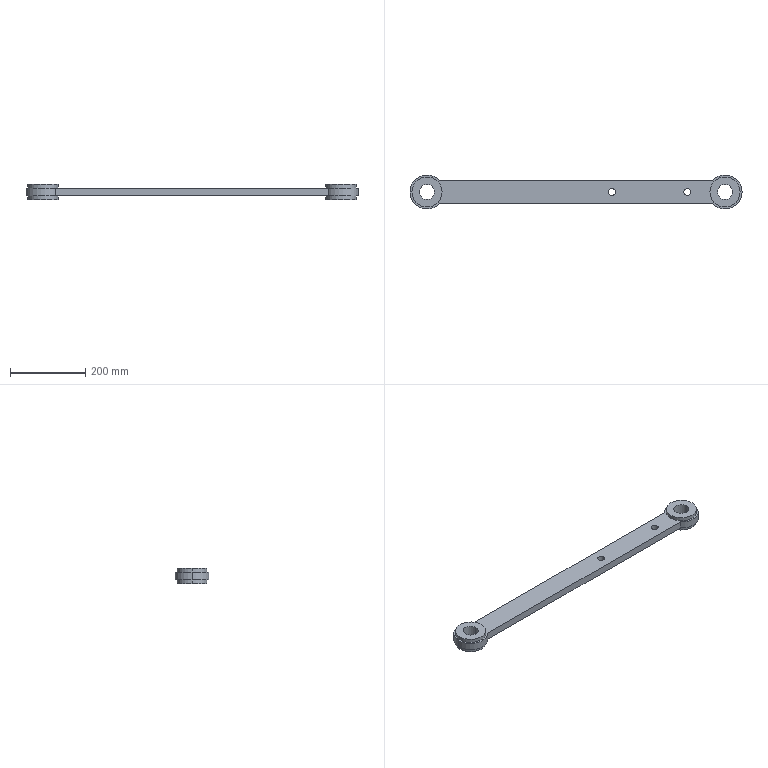Part | SolidWorks | features ICE 2, Extrusion 1, HoleWzd 1 | 1 solid | 27 faces | box 880 x 90 x 40 mm | volume 1192302 mm3 | cylinder 19 | plane 8 | commonest cylinder face diameters 80 x8 19 x4 40 x4 90 x3
STEP:
#1=CARTESIAN_POINT('',(85.5,0.,0.));
#2=VERTEX_POINT('',#1);
#3=CARTESIAN_POINT('',(104.5,0.,0.));
#4=VERTEX_POINT('',#3);
#5=CARTESIAN_POINT('',(95.,0.,0.));
#6=DIRECTION('',(0.,0.,1.));
#7=DIRECTION('',(1.,0.,0.));
#8=AXIS2_PLACEMENT_3D('',#5,#6,#7);
#9=CIRCLE('',#8,9.5);
#10=EDGE_CURVE('',#2,#4,#9,.T.);
#11=ORIENTED_EDGE('',*,*,#10,.F.);
#12=CARTESIAN_POINT('',(85.5,0.,20.));
#13=VERTEX_POINT('',#12);
#14=CARTESIAN_POINT('',(85.5,0.,20.));
#15=DIRECTION('',(0.,0.,1.));
#16=VECTOR('',#15,1000.);
#17=LINE('',#14,#16);
#18=EDGE_CURVE('',#2,#13,#17,.T.);
#19=ORIENTED_EDGE('',*,*,#18,.T.);
#20=CARTESIAN_POINT('',(104.5,0.,20.));
#21=VERTEX_POINT('',#20);
#22=CARTESIAN_POINT('',(95.,0.,20.));
#23=DIRECTION('',(0.,0.,1.));
#24=DIRECTION('',(1.,0.,0.));
#25=AXIS2_PLACEMENT_3D('',#22,#23,#24);
#26=CIRCLE('',#25,9.5);
#27=EDGE_CURVE('',#13,#21,#26,.T.);
#28=ORIENTED_EDGE('',*,*,#27,.T.);
#29=CARTESIAN_POINT('',(104.5,0.,20.));
#30=DIRECTION('',(0.,0.,1.));
#31=VECTOR('',#30,1000.);
#32=LINE('',#29,#31);
#33=EDGE_CURVE('',#4,#21,#32,.T.);
#34=ORIENTED_EDGE('',*,*,#33,.F.);
#35=EDGE_LOOP('',(#11,#19,#28,#34));
#36=FACE_OUTER_BOUND('',#35,.T.);
#37=CARTESIAN_POINT('',(95.,0.,20.));
#38=DIRECTION('',(0.,0.,1.));
#39=DIRECTION('',(1.,0.,0.));
#40=AXIS2_PLACEMENT_3D('',#37,#38,#39);
#41=CYLINDRICAL_SURFACE('',#40,9.5);
#42=ADVANCED_FACE('',(#36),#41,.F.);
#43=CARTESIAN_POINT('',(285.5,0.,0.));
#44=VERTEX_POINT('',#43);
#45=CARTESIAN_POINT('',(304.5,0.,0.));
#46=VERTEX_POINT('',#45);
#47=CARTESIAN_POINT('',(295.,0.,0.));
#48=DIRECTION('',(0.,0.,1.));
#49=DIRECTION('',(1.,0.,0.));
#50=AXIS2_PLACEMENT_3D('',#47,#48,#49);
#51=CIRCLE('',#50,9.5);
#52=EDGE_CURVE('',#44,#46,#51,.T.);
#53=ORIENTED_EDGE('',*,*,#52,.F.);
#54=CARTESIAN_POINT('',(285.5,0.,20.));
#55=VERTEX_POINT('',#54);
#56=CARTESIAN_POINT('',(285.5,0.,20.));
#57=DIRECTION('',(0.,0.,1.));
#58=VECTOR('',#57,1000.);
#59=LINE('',#56,#58);
#60=EDGE_CURVE('',#44,#55,#59,.T.);
#61=ORIENTED_EDGE('',*,*,#60,.T.);
#62=CARTESIAN_POINT('',(304.5,0.,20.));
#63=VERTEX_POINT('',#62);
#64=CARTESIAN_POINT('',(295.,0.,20.));
#65=DIRECTION('',(0.,0.,1.));
#66=DIRECTION('',(1.,0.,0.));
#67=AXIS2_PLACEMENT_3D('',#64,#65,#66);
#68=CIRCLE('',#67,9.5);
#69=EDGE_CURVE('',#55,#63,#68,.T.);
#70=ORIENTED_EDGE('',*,*,#69,.T.);
#71=CARTESIAN_POINT('',(304.5,0.,20.));
#72=DIRECTION('',(0.,0.,1.));
#73=VECTOR('',#72,1000.);
#74=LINE('',#71,#73);
#75=EDGE_CURVE('',#46,#63,#74,.T.);
#76=ORIENTED_EDGE('',*,*,#75,.F.);
#77=EDGE_LOOP('',(#53,#61,#70,#76));
#78=FACE_OUTER_BOUND('',#77,.T.);
#79=CARTESIAN_POINT('',(295.,0.,20.));
#80=DIRECTION('',(0.,0.,1.));
#81=DIRECTION('',(1.,0.,0.));
#82=AXIS2_PLACEMENT_3D('',#79,#80,#81);
#83=CYLINDRICAL_SURFACE('',#82,9.5);
#84=ADVANCED_FACE('',(#78),#83,.F.);
#85=CARTESIAN_POINT('',(-435.,0.,-10.));
#86=VERTEX_POINT('',#85);
#87=CARTESIAN_POINT('',(-355.,0.,-10.));
#88=VERTEX_POINT('',#87);
#89=CARTESIAN_POINT('',(-395.,0.,-10.));
#90=DIRECTION('',(0.,0.,-1.));
#91=DIRECTION('',(-1.,0.,0.));
#92=AXIS2_PLACEMENT_3D('',#89,#90,#91);
#93=CIRCLE('',#92,40.);
#94=EDGE_CURVE('',#86,#88,#93,.T.);
#95=ORIENTED_EDGE('',*,*,#94,.F.);
#96=CARTESIAN_POINT('',(-435.,0.,0.));
#97=VERTEX_POINT('',#96);
#98=CARTESIAN_POINT('',(-435.,0.,-10.));
#99=DIRECTION('',(0.,0.,1.));
#100=VECTOR('',#99,1000.);
#101=LINE('',#98,#100);
#102=EDGE_CURVE('',#86,#97,#101,.T.);
#103=ORIENTED_EDGE('',*,*,#102,.T.);
#104=CARTESIAN_POINT('',(-355.,0.,0.));
#105=VERTEX_POINT('',#104);
#106=CARTESIAN_POINT('',(-395.,0.,0.));
#107=DIRECTION('',(0.,0.,-1.));
#108=DIRECTION('',(1.,0.,0.));
#109=AXIS2_PLACEMENT_3D('',#106,#107,#108);
#110=CIRCLE('',#109,40.);
#111=EDGE_CURVE('',#97,#105,#110,.T.);
#112=ORIENTED_EDGE('',*,*,#111,.T.);
#113=CARTESIAN_POINT('',(-355.,0.,-10.));
#114=DIRECTION('',(0.,0.,1.));
#115=VECTOR('',#114,1000.);
#116=LINE('',#113,#115);
#117=EDGE_CURVE('',#88,#105,#116,.T.);
#118=ORIENTED_EDGE('',*,*,#117,.F.);
#119=EDGE_LOOP('',(#95,#103,#112,#118));
#120=FACE_OUTER_BOUND('',#119,.T.);
#121=CARTESIAN_POINT('',(-395.,0.,-10.));
#122=DIRECTION('',(0.,0.,1.));
#123=DIRECTION('',(1.,0.,0.));
#124=AXIS2_PLACEMENT_3D('',#121,#122,#123);
#125=CYLINDRICAL_SURFACE('',#124,40.);
#126=ADVANCED_FACE('',(#120),#125,.T.);
#127=CARTESIAN_POINT('',(355.,0.,-10.));
#128=VERTEX_POINT('',#127);
#129=CARTESIAN_POINT('',(435.,0.,-10.));
#130=VERTEX_POINT('',#129);
#131=CARTESIAN_POINT('',(395.,0.,-10.));
#132=DIRECTION('',(0.,0.,-1.));
#133=DIRECTION('',(-1.,0.,0.));
#134=AXIS2_PLACEMENT_3D('',#131,#132,#133);
#135=CIRCLE('',#134,40.);
#136=EDGE_CURVE('',#128,#130,#135,.T.);
#137=ORIENTED_EDGE('',*,*,#136,.F.);
#138=CARTESIAN_POINT('',(355.,0.,0.));
#139=VERTEX_POINT('',#138);
#140=CARTESIAN_POINT('',(355.,0.,-10.));
#141=DIRECTION('',(0.,0.,1.));
#142=VECTOR('',#141,1000.);
#143=LINE('',#140,#142);
#144=EDGE_CURVE('',#128,#139,#143,.T.);
#145=ORIENTED_EDGE('',*,*,#144,.T.);
#146=CARTESIAN_POINT('',(435.,0.,0.));
#147=VERTEX_POINT('',#146);
#148=CARTESIAN_POINT('',(395.,0.,0.));
#149=DIRECTION('',(0.,0.,-1.));
#150=DIRECTION('',(-1.,0.,0.));
#151=AXIS2_PLACEMENT_3D('',#148,#149,#150);
#152=CIRCLE('',#151,40.);
#153=EDGE_CURVE('',#139,#147,#152,.T.);
#154=ORIENTED_EDGE('',*,*,#153,.T.);
#155=CARTESIAN_POINT('',(435.,0.,-10.));
#156=DIRECTION('',(0.,0.,1.));
#157=VECTOR('',#156,1000.);
#158=LINE('',#155,#157);
#159=EDGE_CURVE('',#130,#147,#158,.T.);
#160=ORIENTED_EDGE('',*,*,#159,.F.);
#161=EDGE_LOOP('',(#137,#145,#154,#160));
#162=FACE_OUTER_BOUND('',#161,.T.);
#163=CARTESIAN_POINT('',(395.,0.,-10.));
#164=DIRECTION('',(0.,0.,1.));
#165=DIRECTION('',(1.,0.,0.));
#166=AXIS2_PLACEMENT_3D('',#163,#164,#165);
#167=CYLINDRICAL_SURFACE('',#166,40.);
#168=ADVANCED_FACE('',(#162),#167,.T.);
#169=CARTESIAN_POINT('',(435.,0.,30.));
#170=VERTEX_POINT('',#169);
#171=CARTESIAN_POINT('',(355.,0.,30.));
#172=VERTEX_POINT('',#171);
#173=CARTESIAN_POINT('',(395.,0.,30.));
#174=DIRECTION('',(0.,0.,1.));
#175=DIRECTION('',(-1.,0.,0.));
#176=AXIS2_PLACEMENT_3D('',#173,#174,#175);
#177=CIRCLE('',#176,40.);
#178=EDGE_CURVE('',#170,#172,#177,.T.);
#179=ORIENTED_EDGE('',*,*,#178,.F.);
#180=CARTESIAN_POINT('',(435.,0.,20.));
#181=VERTEX_POINT('',#180);
#182=CARTESIAN_POINT('',(435.,0.,30.));
#183=DIRECTION('',(0.,0.,-1.));
#184=VECTOR('',#183,1000.);
#185=LINE('',#182,#184);
#186=EDGE_CURVE('',#170,#181,#185,.T.);
#187=ORIENTED_EDGE('',*,*,#186,.T.);
#188=CARTESIAN_POINT('',(355.,0.,20.));
#189=VERTEX_POINT('',#188);
#190=CARTESIAN_POINT('',(395.,0.,20.));
#191=DIRECTION('',(0.,0.,1.));
#192=DIRECTION('',(-1.,0.,0.));
#193=AXIS2_PLACEMENT_3D('',#190,#191,#192);
#194=CIRCLE('',#193,40.);
#195=EDGE_CURVE('',#181,#189,#194,.T.);
#196=ORIENTED_EDGE('',*,*,#195,.T.);
#197=CARTESIAN_POINT('',(355.,0.,30.));
#198=DIRECTION('',(0.,0.,-1.));
#199=VECTOR('',#198,1000.);
#200=LINE('',#197,#199);
#201=EDGE_CURVE('',#172,#189,#200,.T.);
#202=ORIENTED_EDGE('',*,*,#201,.F.);
#203=EDGE_LOOP('',(#179,#187,#196,#202));
#204=FACE_OUTER_BOUND('',#203,.T.);
#205=CARTESIAN_POINT('',(395.,0.,30.));
#206=DIRECTION('',(0.,0.,-1.));
#207=DIRECTION('',(-1.,0.,0.));
#208=AXIS2_PLACEMENT_3D('',#205,#206,#207);
#209=CYLINDRICAL_SURFACE('',#208,40.);
#210=ADVANCED_FACE('',(#204),#209,.T.);
#211=CARTESIAN_POINT('',(-355.,0.,30.));
#212=VERTEX_POINT('',#211);
#213=CARTESIAN_POINT('',(-435.,0.,30.));
#214=VERTEX_POINT('',#213);
#215=CARTESIAN_POINT('',(-395.,0.,30.));
#216=DIRECTION('',(0.,0.,1.));
#217=DIRECTION('',(1.,0.,0.));
#218=AXIS2_PLACEMENT_3D('',#215,#216,#217);
#219=CIRCLE('',#218,40.);
#220=EDGE_CURVE('',#212,#214,#219,.T.);
#221=ORIENTED_EDGE('',*,*,#220,.F.);
#222=CARTESIAN_POINT('',(-355.,0.,20.));
#223=VERTEX_POINT('',#222);
#224=CARTESIAN_POINT('',(-355.,0.,30.));
#225=DIRECTION('',(0.,0.,-1.));
#226=VECTOR('',#225,1000.);
#227=LINE('',#224,#226);
#228=EDGE_CURVE('',#212,#223,#227,.T.);
#229=ORIENTED_EDGE('',*,*,#228,.T.);
#230=CARTESIAN_POINT('',(-435.,0.,20.));
#231=VERTEX_POINT('',#230);
#232=CARTESIAN_POINT('',(-395.,0.,20.));
#233=DIRECTION('',(0.,0.,1.));
#234=DIRECTION('',(1.,0.,0.));
#235=AXIS2_PLACEMENT_3D('',#232,#233,#234);
#236=CIRCLE('',#235,40.);
#237=EDGE_CURVE('',#223,#231,#236,.T.);
#238=ORIENTED_EDGE('',*,*,#237,.T.);
#239=CARTESIAN_POINT('',(-435.,0.,30.));
#240=DIRECTION('',(0.,0.,-1.));
#241=VECTOR('',#240,1000.);
#242=LINE('',#239,#241);
#243=EDGE_CURVE('',#214,#231,#242,.T.);
#244=ORIENTED_EDGE('',*,*,#243,.F.);
#245=EDGE_LOOP('',(#221,#229,#238,#244));
#246=FACE_OUTER_BOUND('',#245,.T.);
#247=CARTESIAN_POINT('',(-395.,0.,30.));
#248=DIRECTION('',(0.,0.,-1.));
#249=DIRECTION('',(-1.,0.,0.));
#250=AXIS2_PLACEMENT_3D('',#247,#248,#249);
#251=CYLINDRICAL_SURFACE('',#250,40.);
#252=ADVANCED_FACE('',(#246),#251,.T.);
#253=CARTESIAN_POINT('',(-415.,0.,30.));
#254=VERTEX_POINT('',#253);
#255=CARTESIAN_POINT('',(-375.,0.,30.));
#256=VERTEX_POINT('',#255);
#257=CARTESIAN_POINT('',(-395.,0.,30.));
#258=DIRECTION('',(0.,0.,1.));
#259=DIRECTION('',(1.,0.,0.));
#260=AXIS2_PLACEMENT_3D('',#257,#258,#259);
#261=CIRCLE('',#260,20.);
#262=EDGE_CURVE('',#254,#256,#261,.T.);
#263=ORIENTED_EDGE('',*,*,#262,.T.);
#264=CARTESIAN_POINT('',(-375.,0.,-10.));
#265=VERTEX_POINT('',#264);
#266=CARTESIAN_POINT('',(-375.,0.,20.));
#267=DIRECTION('',(0.,0.,-1.));
#268=VECTOR('',#267,1000.);
#269=LINE('',#266,#268);
#270=EDGE_CURVE('',#256,#265,#269,.T.);
#271=ORIENTED_EDGE('',*,*,#270,.T.);
#272=CARTESIAN_POINT('',(-415.,0.,-10.));
#273=VERTEX_POINT('',#272);
#274=CARTESIAN_POINT('',(-395.,0.,-10.));
#275=DIRECTION('',(0.,0.,-1.));
#276=DIRECTION('',(-1.,0.,0.));
#277=AXIS2_PLACEMENT_3D('',#274,#275,#276);
#278=CIRCLE('',#277,20.);
#279=EDGE_CURVE('',#265,#273,#278,.T.);
#280=ORIENTED_EDGE('',*,*,#279,.T.);
#281=CARTESIAN_POINT('',(-415.,0.,20.));
#282=DIRECTION('',(0.,0.,-1.));
#283=VECTOR('',#282,1000.);
#284=LINE('',#281,#283);
#285=EDGE_CURVE('',#254,#273,#284,.T.);
#286=ORIENTED_EDGE('',*,*,#285,.F.);
#287=EDGE_LOOP('',(#263,#271,#280,#286));
#288=FACE_OUTER_BOUND('',#287,.T.);
#289=CARTESIAN_POINT('',(-395.,0.,20.));
#290=DIRECTION('',(0.,0.,-1.));
#291=DIRECTION('',(-1.,0.,0.));
#292=AXIS2_PLACEMENT_3D('',#289,#290,#291);
#293=CYLINDRICAL_SURFACE('',#292,20.);
#294=ADVANCED_FACE('',(#288),#293,.F.);
#295=CARTESIAN_POINT('',(375.,0.,30.));
#296=VERTEX_POINT('',#295);
#297=CARTESIAN_POINT('',(415.,0.,30.));
#298=VERTEX_POINT('',#297);
#299=CARTESIAN_POINT('',(395.,0.,30.));
#300=DIRECTION('',(0.,0.,1.));
#301=DIRECTION('',(-1.,0.,0.));
#302=AXIS2_PLACEMENT_3D('',#299,#300,#301);
#303=CIRCLE('',#302,20.);
#304=EDGE_CURVE('',#296,#298,#303,.T.);
#305=ORIENTED_EDGE('',*,*,#304,.T.);
#306=CARTESIAN_POINT('',(415.,0.,-10.));
#307=VERTEX_POINT('',#306);
#308=CARTESIAN_POINT('',(415.,0.,20.));
#309=DIRECTION('',(0.,0.,-1.));
#310=VECTOR('',#309,1000.);
#311=LINE('',#308,#310);
#312=EDGE_CURVE('',#298,#307,#311,.T.);
#313=ORIENTED_EDGE('',*,*,#312,.T.);
#314=CARTESIAN_POINT('',(375.,0.,-10.));
#315=VERTEX_POINT('',#314);
#316=CARTESIAN_POINT('',(395.,0.,-10.));
#317=DIRECTION('',(0.,0.,-1.));
#318=DIRECTION('',(-1.,0.,0.));
#319=AXIS2_PLACEMENT_3D('',#316,#317,#318);
#320=CIRCLE('',#319,20.);
#321=EDGE_CURVE('',#307,#315,#320,.T.);
#322=ORIENTED_EDGE('',*,*,#321,.T.);
#323=CARTESIAN_POINT('',(375.,0.,20.));
#324=DIRECTION('',(0.,0.,-1.));
#325=VECTOR('',#324,1000.);
#326=LINE('',#323,#325);
#327=EDGE_CURVE('',#296,#315,#326,.T.);
#328=ORIENTED_EDGE('',*,*,#327,.F.);
#329=EDGE_LOOP('',(#305,#313,#322,#328));
#330=FACE_OUTER_BOUND('',#329,.T.);
#331=CARTESIAN_POINT('',(395.,0.,20.));
#332=DIRECTION('',(0.,0.,-1.));
#333=DIRECTION('',(-1.,0.,0.));
#334=AXIS2_PLACEMENT_3D('',#331,#332,#333);
#335=CYLINDRICAL_SURFACE('',#334,20.);
#336=ADVANCED_FACE('',(#330),#335,.F.);
#337=CARTESIAN_POINT('',(-440.,0.,20.));
#338=VERTEX_POINT('',#337);
#339=CARTESIAN_POINT('',(-361.459,-30.,20.));
#340=VERTEX_POINT('',#339);
#341=CARTESIAN_POINT('',(-395.,0.,20.));
#342=DIRECTION('',(0.,0.,1.));
#343=DIRECTION('',(1.,0.,0.));
#344=AXIS2_PLACEMENT_3D('',#341,#342,#343);
#345=CIRCLE('',#344,45.);
#346=EDGE_CURVE('',#338,#340,#345,.T.);
#347=ORIENTED_EDGE('',*,*,#346,.F.);
#348=CARTESIAN_POINT('',(-440.,0.,0.));
#349=VERTEX_POINT('',#348);
#350=CARTESIAN_POINT('',(-440.,0.,20.));
#351=DIRECTION('',(0.,0.,-1.));
#352=VECTOR('',#351,1000.);
#353=LINE('',#350,#352);
#354=EDGE_CURVE('',#338,#349,#353,.T.);
#355=ORIENTED_EDGE('',*,*,#354,.T.);
#356=CARTESIAN_POINT('',(-361.459,-30.,0.));
#357=VERTEX_POINT('',#356);
#358=CARTESIAN_POINT('',(-395.,0.,0.));
#359=DIRECTION('',(0.,0.,1.));
#360=DIRECTION('',(1.,0.,0.));
#361=AXIS2_PLACEMENT_3D('',#358,#359,#360);
#362=CIRCLE('',#361,45.);
#363=EDGE_CURVE('',#349,#357,#362,.T.);
#364=ORIENTED_EDGE('',*,*,#363,.T.);
#365=CARTESIAN_POINT('',(-361.459,-30.,20.));
#366=DIRECTION('',(0.,0.,-1.));
#367=VECTOR('',#366,1000.);
#368=LINE('',#365,#367);
#369=EDGE_CURVE('',#340,#357,#368,.T.);
#370=ORIENTED_EDGE('',*,*,#369,.F.);
#371=EDGE_LOOP('',(#347,#355,#364,#370));
#372=FACE_OUTER_BOUND('',#371,.T.);
#373=CARTESIAN_POINT('',(-395.,0.,20.));
#374=DIRECTION('',(0.,0.,-1.));
#375=DIRECTION('',(-1.,0.,0.));
#376=AXIS2_PLACEMENT_3D('',#373,#374,#375);
#377=CYLINDRICAL_SURFACE('',#376,45.);
#378=ADVANCED_FACE('',(#372),#377,.T.);
#379=CARTESIAN_POINT('',(95.,0.,0.));
#380=DIRECTION('',(0.,0.,1.));
#381=DIRECTION('',(1.,0.,0.));
#382=AXIS2_PLACEMENT_3D('',#379,#380,#381);
#383=CIRCLE('',#382,9.5);
#384=EDGE_CURVE('',#4,#2,#383,.T.);
#385=ORIENTED_EDGE('',*,*,#384,.T.);
#386=ORIENTED_EDGE('',*,*,#10,.T.);
#387=EDGE_LOOP('',(#385,#386));
#388=FACE_BOUND('',#387,.T.);
#389=CARTESIAN_POINT('',(295.,0.,0.));
#390=DIRECTION('',(0.,0.,1.));
#391=DIRECTION('',(1.,0.,0.));
#392=AXIS2_PLACEMENT_3D('',#389,#390,#391);
#393=CIRCLE('',#392,9.5);
#394=EDGE_CURVE('',#46,#44,#393,.T.);
#395=ORIENTED_EDGE('',*,*,#394,.T.);
#396=ORIENTED_EDGE('',*,*,#52,.T.);
#397=EDGE_LOOP('',(#395,#396));
#398=FACE_BOUND('',#397,.T.);
#399=CARTESIAN_POINT('',(361.459,-30.,0.));
#400=VERTEX_POINT('',#399);
#401=CARTESIAN_POINT('',(361.459,30.,0.));
#402=VERTEX_POINT('',#401);
#403=CARTESIAN_POINT('',(395.,0.,0.));
#404=DIRECTION('',(0.,0.,1.));
#405=DIRECTION('',(1.,0.,0.));
#406=AXIS2_PLACEMENT_3D('',#403,#404,#405);
#407=CIRCLE('',#406,45.);
#408=EDGE_CURVE('',#400,#402,#407,.T.);
#409=ORIENTED_EDGE('',*,*,#408,.F.);
#410=CARTESIAN_POINT('',(0.,-30.,0.));
#411=DIRECTION('',(-1.,0.,0.));
#412=VECTOR('',#411,1000.);
#413=LINE('',#410,#412);
#414=EDGE_CURVE('',#400,#357,#413,.T.);
#415=ORIENTED_EDGE('',*,*,#414,.T.);
#416=ORIENTED_EDGE('',*,*,#363,.F.);
#417=CARTESIAN_POINT('',(-361.459,30.,0.));
#418=VERTEX_POINT('',#417);
#419=CARTESIAN_POINT('',(-395.,0.,0.));
#420=DIRECTION('',(0.,0.,1.));
#421=DIRECTION('',(1.,0.,0.));
#422=AXIS2_PLACEMENT_3D('',#419,#420,#421);
#423=CIRCLE('',#422,45.);
#424=EDGE_CURVE('',#418,#349,#423,.T.);
#425=ORIENTED_EDGE('',*,*,#424,.F.);
#426=CARTESIAN_POINT('',(0.,30.,0.));
#427=DIRECTION('',(-1.,0.,0.));
#428=VECTOR('',#427,1000.);
#429=LINE('',#426,#428);
#430=EDGE_CURVE('',#402,#418,#429,.T.);
#431=ORIENTED_EDGE('',*,*,#430,.F.);
#432=EDGE_LOOP('',(#409,#415,#416,#425,#431));
#433=FACE_OUTER_BOUND('',#432,.T.);
#434=CARTESIAN_POINT('',(395.,0.,0.));
#435=DIRECTION('',(0.,0.,-1.));
#436=DIRECTION('',(-1.,0.,0.));
#437=AXIS2_PLACEMENT_3D('',#434,#435,#436);
#438=CIRCLE('',#437,40.);
#439=EDGE_CURVE('',#147,#139,#438,.T.);
#440=ORIENTED_EDGE('',*,*,#439,.F.);
#441=ORIENTED_EDGE('',*,*,#153,.F.);
#442=EDGE_LOOP('',(#440,#441));
#443=FACE_BOUND('',#442,.T.);
#444=CARTESIAN_POINT('',(-395.,0.,0.));
#445=DIRECTION('',(0.,0.,-1.));
#446=DIRECTION('',(1.,0.,0.));
#447=AXIS2_PLACEMENT_3D('',#444,#445,#446);
#448=CIRCLE('',#447,40.);
#449=EDGE_CURVE('',#105,#97,#448,.T.);
#450=ORIENTED_EDGE('',*,*,#449,.F.);
#451=ORIENTED_EDGE('',*,*,#111,.F.);
#452=EDGE_LOOP('',(#450,#451));
#453=FACE_BOUND('',#452,.T.);
#454=CARTESIAN_POINT('',(0.,0.,0.));
#455=DIRECTION('',(0.,0.,1.));
#456=DIRECTION('',(1.,0.,0.));
#457=AXIS2_PLACEMENT_3D('',#454,#455,#456);
#458=PLANE('',#457);
#459=ADVANCED_FACE('',(#388,#398,#433,#443,#453),#458,.F.);
#460=CARTESIAN_POINT('',(95.,0.,20.));
#461=DIRECTION('',(0.,0.,1.));
#462=DIRECTION('',(1.,0.,0.));
#463=AXIS2_PLACEMENT_3D('',#460,#461,#462);
#464=CIRCLE('',#463,9.5);
#465=EDGE_CURVE('',#21,#13,#464,.T.);
#466=ORIENTED_EDGE('',*,*,#465,.F.);
#467=ORIENTED_EDGE('',*,*,#27,.F.);
#468=EDGE_LOOP('',(#466,#467));
#469=FACE_BOUND('',#468,.T.);
#470=CARTESIAN_POINT('',(295.,0.,20.));
#471=DIRECTION('',(0.,0.,1.));
#472=DIRECTION('',(1.,0.,0.));
#473=AXIS2_PLACEMENT_3D('',#470,#471,#472);
#474=CIRCLE('',#473,9.5);
#475=EDGE_CURVE('',#63,#55,#474,.T.);
#476=ORIENTED_EDGE('',*,*,#475,.F.);
#477=ORIENTED_EDGE('',*,*,#69,.F.);
#478=EDGE_LOOP('',(#476,#477));
#479=FACE_BOUND('',#478,.T.);
#480=CARTESIAN_POINT('',(-395.,0.,20.));
#481=DIRECTION('',(0.,0.,1.));
#482=DIRECTION('',(1.,0.,0.));
#483=AXIS2_PLACEMENT_3D('',#480,#481,#482);
#484=CIRCLE('',#483,40.);
#485=EDGE_CURVE('',#231,#223,#484,.T.);
#486=ORIENTED_EDGE('',*,*,#485,.F.);
#487=ORIENTED_EDGE('',*,*,#237,.F.);
#488=EDGE_LOOP('',(#486,#487));
#489=FACE_BOUND('',#488,.T.);
#490=CARTESIAN_POINT('',(361.459,-30.,20.));
#491=VERTEX_POINT('',#490);
#492=CARTESIAN_POINT('',(361.459,30.,20.));
#493=VERTEX_POINT('',#492);
#494=CARTESIAN_POINT('',(395.,0.,20.));
#495=DIRECTION('',(0.,0.,1.));
#496=DIRECTION('',(1.,0.,0.));
#497=AXIS2_PLACEMENT_3D('',#494,#495,#496);
#498=CIRCLE('',#497,45.);
#499=EDGE_CURVE('',#491,#493,#498,.T.);
#500=ORIENTED_EDGE('',*,*,#499,.T.);
#501=CARTESIAN_POINT('',(-361.459,30.,20.));
#502=VERTEX_POINT('',#501);
#503=CARTESIAN_POINT('',(0.,30.,20.));
#504=DIRECTION('',(-1.,0.,0.));
#505=VECTOR('',#504,1000.);
#506=LINE('',#503,#505);
#507=EDGE_CURVE('',#493,#502,#506,.T.);
#508=ORIENTED_EDGE('',*,*,#507,.T.);
#509=CARTESIAN_POINT('',(-395.,0.,20.));
#510=DIRECTION('',(0.,0.,1.));
#511=DIRECTION('',(1.,0.,0.));
#512=AXIS2_PLACEMENT_3D('',#509,#510,#511);
#513=CIRCLE('',#512,45.);
#514=EDGE_CURVE('',#502,#338,#513,.T.);
#515=ORIENTED_EDGE('',*,*,#514,.T.);
#516=ORIENTED_EDGE('',*,*,#346,.T.);
#517=CARTESIAN_POINT('',(0.,-30.,20.));
#518=DIRECTION('',(-1.,0.,0.));
#519=VECTOR('',#518,1000.);
#520=LINE('',#517,#519);
#521=EDGE_CURVE('',#491,#340,#520,.T.);
#522=ORIENTED_EDGE('',*,*,#521,.F.);
#523=EDGE_LOOP('',(#500,#508,#515,#516,#522));
#524=FACE_OUTER_BOUND('',#523,.T.);
#525=CARTESIAN_POINT('',(395.,0.,20.));
#526=DIRECTION('',(0.,0.,1.));
#527=DIRECTION('',(-1.,0.,0.));
#528=AXIS2_PLACEMENT_3D('',#525,#526,#527);
#529=CIRCLE('',#528,40.);
#530=EDGE_CURVE('',#189,#181,#529,.T.);
#531=ORIENTED_EDGE('',*,*,#530,.F.);
#532=ORIENTED_EDGE('',*,*,#195,.F.);
#533=EDGE_LOOP('',(#531,#532));
#534=FACE_BOUND('',#533,.T.);
#535=CARTESIAN_POINT('',(0.,0.,20.));
#536=DIRECTION('',(0.,0.,1.));
#537=DIRECTION('',(1.,0.,0.));
#538=AXIS2_PLACEMENT_3D('',#535,#536,#537);
#539=PLANE('',#538);
#540=ADVANCED_FACE('',(#469,#479,#489,#524,#534),#539,.T.);
#541=ORIENTED_EDGE('',*,*,#408,.T.);
#542=CARTESIAN_POINT('',(361.459,30.,20.));
#543=DIRECTION('',(0.,0.,-1.));
#544=VECTOR('',#543,1000.);
#545=LINE('',#542,#544);
#546=EDGE_CURVE('',#493,#402,#545,.T.);
#547=ORIENTED_EDGE('',*,*,#546,.F.);
#548=ORIENTED_EDGE('',*,*,#499,.F.);
#549=CARTESIAN_POINT('',(361.459,-30.,20.));
#550=DIRECTION('',(0.,0.,-1.));
#551=VECTOR('',#550,1000.);
#552=LINE('',#549,#551);
#553=EDGE_CURVE('',#491,#400,#552,.T.);
#554=ORIENTED_EDGE('',*,*,#553,.T.);
#555=EDGE_LOOP('',(#541,#547,#548,#554));
#556=FACE_OUTER_BOUND('',#555,.T.);
#557=CARTESIAN_POINT('',(395.,0.,20.));
#558=DIRECTION('',(0.,0.,-1.));
#559=DIRECTION('',(-1.,0.,0.));
#560=AXIS2_PLACEMENT_3D('',#557,#558,#559);
#561=CYLINDRICAL_SURFACE('',#560,45.);
#562=ADVANCED_FACE('',(#556),#561,.T.);
#563=ORIENTED_EDGE('',*,*,#430,.T.);
#564=CARTESIAN_POINT('',(-361.459,30.,20.));
#565=DIRECTION('',(0.,0.,-1.));
#566=VECTOR('',#565,1000.);
#567=LINE('',#564,#566);
#568=EDGE_CURVE('',#502,#418,#567,.T.);
#569=ORIENTED_EDGE('',*,*,#568,.F.);
#570=ORIENTED_EDGE('',*,*,#507,.F.);
#571=ORIENTED_EDGE('',*,*,#546,.T.);
#572=EDGE_LOOP('',(#563,#569,#570,#571));
#573=FACE_OUTER_BOUND('',#572,.T.);
#574=CARTESIAN_POINT('',(0.,30.,20.));
#575=DIRECTION('',(0.,-1.,0.));
#576=DIRECTION('',(1.,0.,0.));
#577=AXIS2_PLACEMENT_3D('',#574,#575,#576);
#578=PLANE('',#577);
#579=ADVANCED_FACE('',(#573),#578,.F.);
#580=ORIENTED_EDGE('',*,*,#354,.F.);
#581=ORIENTED_EDGE('',*,*,#514,.F.);
#582=ORIENTED_EDGE('',*,*,#568,.T.);
#583=ORIENTED_EDGE('',*,*,#424,.T.);
#584=EDGE_LOOP('',(#580,#581,#582,#583));
#585=FACE_OUTER_BOUND('',#584,.T.);
#586=CARTESIAN_POINT('',(-395.,0.,20.));
#587=DIRECTION('',(0.,0.,-1.));
#588=DIRECTION('',(-1.,0.,0.));
#589=AXIS2_PLACEMENT_3D('',#586,#587,#588);
#590=CYLINDRICAL_SURFACE('',#589,45.);
#591=ADVANCED_FACE('',(#585),#590,.T.);
#592=ORIENTED_EDGE('',*,*,#312,.F.);
#593=CARTESIAN_POINT('',(395.,0.,30.));
#594=DIRECTION('',(0.,0.,1.));
#595=DIRECTION('',(-1.,0.,0.));
#596=AXIS2_PLACEMENT_3D('',#593,#594,#595);
#597=CIRCLE('',#596,20.);
#598=EDGE_CURVE('',#298,#296,#597,.T.);
#599=ORIENTED_EDGE('',*,*,#598,.T.);
#600=ORIENTED_EDGE('',*,*,#327,.T.);
#601=CARTESIAN_POINT('',(395.,0.,-10.));
#602=DIRECTION('',(0.,0.,-1.));
#603=DIRECTION('',(-1.,0.,0.));
#604=AXIS2_PLACEMENT_3D('',#601,#602,#603);
#605=CIRCLE('',#604,20.);
#606=EDGE_CURVE('',#315,#307,#605,.T.);
#607=ORIENTED_EDGE('',*,*,#606,.T.);
#608=EDGE_LOOP('',(#592,#599,#600,#607));
#609=FACE_OUTER_BOUND('',#608,.T.);
#610=CARTESIAN_POINT('',(395.,0.,20.));
#611=DIRECTION('',(0.,0.,-1.));
#612=DIRECTION('',(-1.,0.,0.));
#613=AXIS2_PLACEMENT_3D('',#610,#611,#612);
#614=CYLINDRICAL_SURFACE('',#613,20.);
#615=ADVANCED_FACE('',(#609),#614,.F.);
#616=ORIENTED_EDGE('',*,*,#414,.F.);
#617=ORIENTED_EDGE('',*,*,#553,.F.);
#618=ORIENTED_EDGE('',*,*,#521,.T.);
#619=ORIENTED_EDGE('',*,*,#369,.T.);
#620=EDGE_LOOP('',(#616,#617,#618,#619));
#621=FACE_OUTER_BOUND('',#620,.T.);
#622=CARTESIAN_POINT('',(0.,-30.,20.));
#623=DIRECTION('',(0.,-1.,0.));
#624=DIRECTION('',(1.,0.,0.));
#625=AXIS2_PLACEMENT_3D('',#622,#623,#624);
#626=PLANE('',#625);
#627=ADVANCED_FACE('',(#621),#626,.T.);
#628=ORIENTED_EDGE('',*,*,#270,.F.);
#629=CARTESIAN_POINT('',(-395.,0.,30.));
#630=DIRECTION('',(0.,0.,1.));
#631=DIRECTION('',(1.,0.,0.));
#632=AXIS2_PLACEMENT_3D('',#629,#630,#631);
#633=CIRCLE('',#632,20.);
#634=EDGE_CURVE('',#256,#254,#633,.T.);
#635=ORIENTED_EDGE('',*,*,#634,.T.);
#636=ORIENTED_EDGE('',*,*,#285,.T.);
#637=CARTESIAN_POINT('',(-395.,0.,-10.));
#638=DIRECTION('',(0.,0.,-1.));
#639=DIRECTION('',(-1.,0.,0.));
#640=AXIS2_PLACEMENT_3D('',#637,#638,#639);
#641=CIRCLE('',#640,20.);
#642=EDGE_CURVE('',#273,#265,#641,.T.);
#643=ORIENTED_EDGE('',*,*,#642,.T.);
#644=EDGE_LOOP('',(#628,#635,#636,#643));
#645=FACE_OUTER_BOUND('',#644,.T.);
#646=CARTESIAN_POINT('',(-395.,0.,20.));
#647=DIRECTION('',(0.,0.,-1.));
#648=DIRECTION('',(-1.,0.,0.));
#649=AXIS2_PLACEMENT_3D('',#646,#647,#648);
#650=CYLINDRICAL_SURFACE('',#649,20.);
#651=ADVANCED_FACE('',(#645),#650,.F.);
#652=CARTESIAN_POINT('',(-395.,0.,30.));
#653=DIRECTION('',(0.,0.,1.));
#654=DIRECTION('',(1.,0.,0.));
#655=AXIS2_PLACEMENT_3D('',#652,#653,#654);
#656=CIRCLE('',#655,40.);
#657=EDGE_CURVE('',#214,#212,#656,.T.);
#658=ORIENTED_EDGE('',*,*,#657,.T.);
#659=ORIENTED_EDGE('',*,*,#220,.T.);
#660=EDGE_LOOP('',(#658,#659));
#661=FACE_OUTER_BOUND('',#660,.T.);
#662=ORIENTED_EDGE('',*,*,#262,.F.);
#663=ORIENTED_EDGE('',*,*,#634,.F.);
#664=EDGE_LOOP('',(#662,#663));
#665=FACE_BOUND('',#664,.T.);
#666=CARTESIAN_POINT('',(-395.,0.,30.));
#667=DIRECTION('',(0.,0.,1.));
#668=DIRECTION('',(1.,0.,0.));
#669=AXIS2_PLACEMENT_3D('',#666,#667,#668);
#670=PLANE('',#669);
#671=ADVANCED_FACE('',(#661,#665),#670,.T.);
#672=ORIENTED_EDGE('',*,*,#228,.F.);
#673=ORIENTED_EDGE('',*,*,#657,.F.);
#674=ORIENTED_EDGE('',*,*,#243,.T.);
#675=ORIENTED_EDGE('',*,*,#485,.T.);
#676=EDGE_LOOP('',(#672,#673,#674,#675));
#677=FACE_OUTER_BOUND('',#676,.T.);
#678=CARTESIAN_POINT('',(-395.,0.,30.));
#679=DIRECTION('',(0.,0.,-1.));
#680=DIRECTION('',(-1.,0.,0.));
#681=AXIS2_PLACEMENT_3D('',#678,#679,#680);
#682=CYLINDRICAL_SURFACE('',#681,40.);
#683=ADVANCED_FACE('',(#677),#682,.T.);
#684=CARTESIAN_POINT('',(395.,0.,30.));
#685=DIRECTION('',(0.,0.,1.));
#686=DIRECTION('',(-1.,0.,0.));
#687=AXIS2_PLACEMENT_3D('',#684,#685,#686);
#688=CIRCLE('',#687,40.);
#689=EDGE_CURVE('',#172,#170,#688,.T.);
#690=ORIENTED_EDGE('',*,*,#689,.T.);
#691=ORIENTED_EDGE('',*,*,#178,.T.);
#692=EDGE_LOOP('',(#690,#691));
#693=FACE_OUTER_BOUND('',#692,.T.);
#694=ORIENTED_EDGE('',*,*,#304,.F.);
#695=ORIENTED_EDGE('',*,*,#598,.F.);
#696=EDGE_LOOP('',(#694,#695));
#697=FACE_BOUND('',#696,.T.);
#698=CARTESIAN_POINT('',(395.,0.,30.));
#699=DIRECTION('',(0.,0.,-1.));
#700=DIRECTION('',(-1.,0.,0.));
#701=AXIS2_PLACEMENT_3D('',#698,#699,#700);
#702=PLANE('',#701);
#703=ADVANCED_FACE('',(#693,#697),#702,.F.);
#704=ORIENTED_EDGE('',*,*,#186,.F.);
#705=ORIENTED_EDGE('',*,*,#689,.F.);
#706=ORIENTED_EDGE('',*,*,#201,.T.);
#707=ORIENTED_EDGE('',*,*,#530,.T.);
#708=EDGE_LOOP('',(#704,#705,#706,#707));
#709=FACE_OUTER_BOUND('',#708,.T.);
#710=CARTESIAN_POINT('',(395.,0.,30.));
#711=DIRECTION('',(0.,0.,-1.));
#712=DIRECTION('',(-1.,0.,0.));
#713=AXIS2_PLACEMENT_3D('',#710,#711,#712);
#714=CYLINDRICAL_SURFACE('',#713,40.);
#715=ADVANCED_FACE('',(#709),#714,.T.);
#716=CARTESIAN_POINT('',(395.,0.,-10.));
#717=DIRECTION('',(0.,0.,-1.));
#718=DIRECTION('',(-1.,0.,0.));
#719=AXIS2_PLACEMENT_3D('',#716,#717,#718);
#720=CIRCLE('',#719,40.);
#721=EDGE_CURVE('',#130,#128,#720,.T.);
#722=ORIENTED_EDGE('',*,*,#721,.T.);
#723=ORIENTED_EDGE('',*,*,#136,.T.);
#724=EDGE_LOOP('',(#722,#723));
#725=FACE_OUTER_BOUND('',#724,.T.);
#726=ORIENTED_EDGE('',*,*,#606,.F.);
#727=ORIENTED_EDGE('',*,*,#321,.F.);
#728=EDGE_LOOP('',(#726,#727));
#729=FACE_BOUND('',#728,.T.);
#730=CARTESIAN_POINT('',(395.,0.,-10.));
#731=DIRECTION('',(0.,0.,-1.));
#732=DIRECTION('',(-1.,0.,0.));
#733=AXIS2_PLACEMENT_3D('',#730,#731,#732);
#734=PLANE('',#733);
#735=ADVANCED_FACE('',(#725,#729),#734,.T.);
#736=ORIENTED_EDGE('',*,*,#144,.F.);
#737=ORIENTED_EDGE('',*,*,#721,.F.);
#738=ORIENTED_EDGE('',*,*,#159,.T.);
#739=ORIENTED_EDGE('',*,*,#439,.T.);
#740=EDGE_LOOP('',(#736,#737,#738,#739));
#741=FACE_OUTER_BOUND('',#740,.T.);
#742=CARTESIAN_POINT('',(395.,0.,-10.));
#743=DIRECTION('',(0.,0.,1.));
#744=DIRECTION('',(1.,0.,0.));
#745=AXIS2_PLACEMENT_3D('',#742,#743,#744);
#746=CYLINDRICAL_SURFACE('',#745,40.);
#747=ADVANCED_FACE('',(#741),#746,.T.);
#748=CARTESIAN_POINT('',(-395.,0.,-10.));
#749=DIRECTION('',(0.,0.,-1.));
#750=DIRECTION('',(-1.,0.,0.));
#751=AXIS2_PLACEMENT_3D('',#748,#749,#750);
#752=CIRCLE('',#751,40.);
#753=EDGE_CURVE('',#88,#86,#752,.T.);
#754=ORIENTED_EDGE('',*,*,#753,.T.);
#755=ORIENTED_EDGE('',*,*,#94,.T.);
#756=EDGE_LOOP('',(#754,#755));
#757=FACE_OUTER_BOUND('',#756,.T.);
#758=ORIENTED_EDGE('',*,*,#642,.F.);
#759=ORIENTED_EDGE('',*,*,#279,.F.);
#760=EDGE_LOOP('',(#758,#759));
#761=FACE_BOUND('',#760,.T.);
#762=CARTESIAN_POINT('',(-395.,0.,-10.));
#763=DIRECTION('',(0.,0.,-1.));
#764=DIRECTION('',(-1.,0.,0.));
#765=AXIS2_PLACEMENT_3D('',#762,#763,#764);
#766=PLANE('',#765);
#767=ADVANCED_FACE('',(#757,#761),#766,.T.);
#768=ORIENTED_EDGE('',*,*,#102,.F.);
#769=ORIENTED_EDGE('',*,*,#753,.F.);
#770=ORIENTED_EDGE('',*,*,#117,.T.);
#771=ORIENTED_EDGE('',*,*,#449,.T.);
#772=EDGE_LOOP('',(#768,#769,#770,#771));
#773=FACE_OUTER_BOUND('',#772,.T.);
#774=CARTESIAN_POINT('',(-395.,0.,-10.));
#775=DIRECTION('',(0.,0.,1.));
#776=DIRECTION('',(1.,0.,0.));
#777=AXIS2_PLACEMENT_3D('',#774,#775,#776);
#778=CYLINDRICAL_SURFACE('',#777,40.);
#779=ADVANCED_FACE('',(#773),#778,.T.);
#780=ORIENTED_EDGE('',*,*,#60,.F.);
#781=ORIENTED_EDGE('',*,*,#394,.F.);
#782=ORIENTED_EDGE('',*,*,#75,.T.);
#783=ORIENTED_EDGE('',*,*,#475,.T.);
#784=EDGE_LOOP('',(#780,#781,#782,#783));
#785=FACE_OUTER_BOUND('',#784,.T.);
#786=CARTESIAN_POINT('',(295.,0.,20.));
#787=DIRECTION('',(0.,0.,1.));
#788=DIRECTION('',(1.,0.,0.));
#789=AXIS2_PLACEMENT_3D('',#786,#787,#788);
#790=CYLINDRICAL_SURFACE('',#789,9.5);
#791=ADVANCED_FACE('',(#785),#790,.F.);
#792=ORIENTED_EDGE('',*,*,#18,.F.);
#793=ORIENTED_EDGE('',*,*,#384,.F.);
#794=ORIENTED_EDGE('',*,*,#33,.T.);
#795=ORIENTED_EDGE('',*,*,#465,.T.);
#796=EDGE_LOOP('',(#792,#793,#794,#795));
#797=FACE_OUTER_BOUND('',#796,.T.);
#798=CARTESIAN_POINT('',(95.,0.,20.));
#799=DIRECTION('',(0.,0.,1.));
#800=DIRECTION('',(1.,0.,0.));
#801=AXIS2_PLACEMENT_3D('',#798,#799,#800);
#802=CYLINDRICAL_SURFACE('',#801,9.5);
#803=ADVANCED_FACE('',(#797),#802,.F.);
#804=CLOSED_SHELL('',(#42,#84,#126,#168,#210,#252,#294,#336,#378,#459,#540,#562,#579,#591,#615,#627,#651,#671,#683,#703,#715,#735,#747,#767,#779,#791,#803));
#805=MANIFOLD_SOLID_BREP('',#804);
#806=CARTESIAN_POINT('',(0.,0.,0.));
#807=DIRECTION('',(0.,0.,1.));
#808=DIRECTION('',(1.,0.,0.));
#809=AXIS2_PLACEMENT_3D('',#806,#807,#808);
#810=(LENGTH_UNIT()NAMED_UNIT(*)SI_UNIT(.MILLI.,.METRE.));
#811=UNCERTAINTY_MEASURE_WITH_UNIT(LENGTH_MEASURE(0.00001),#810,'','');
#812=(NAMED_UNIT(*)PLANE_ANGLE_UNIT()SI_UNIT($,.RADIAN.));
#813=(NAMED_UNIT(*)SI_UNIT($,.STERADIAN.)SOLID_ANGLE_UNIT());
#814=(GEOMETRIC_REPRESENTATION_CONTEXT(3)GLOBAL_UNCERTAINTY_ASSIGNED_CONTEXT((#811))GLOBAL_UNIT_ASSIGNED_CONTEXT((#810,#812,#813))REPRESENTATION_CONTEXT('',''));
#815=ADVANCED_BREP_SHAPE_REPRESENTATION('',(#805,#809),#814);